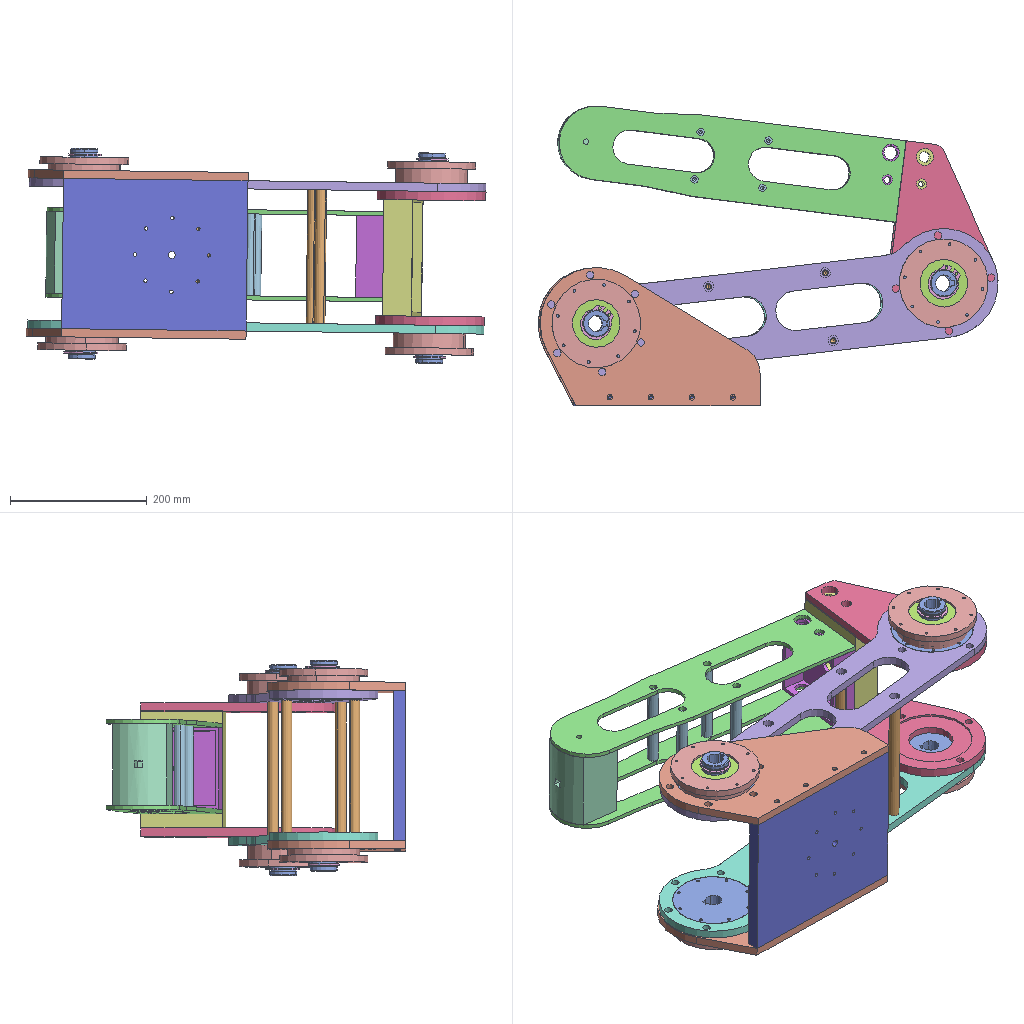Assembly | SolidWorks | 15 different items | 36 placed | box 673 x 438 x 315 mm
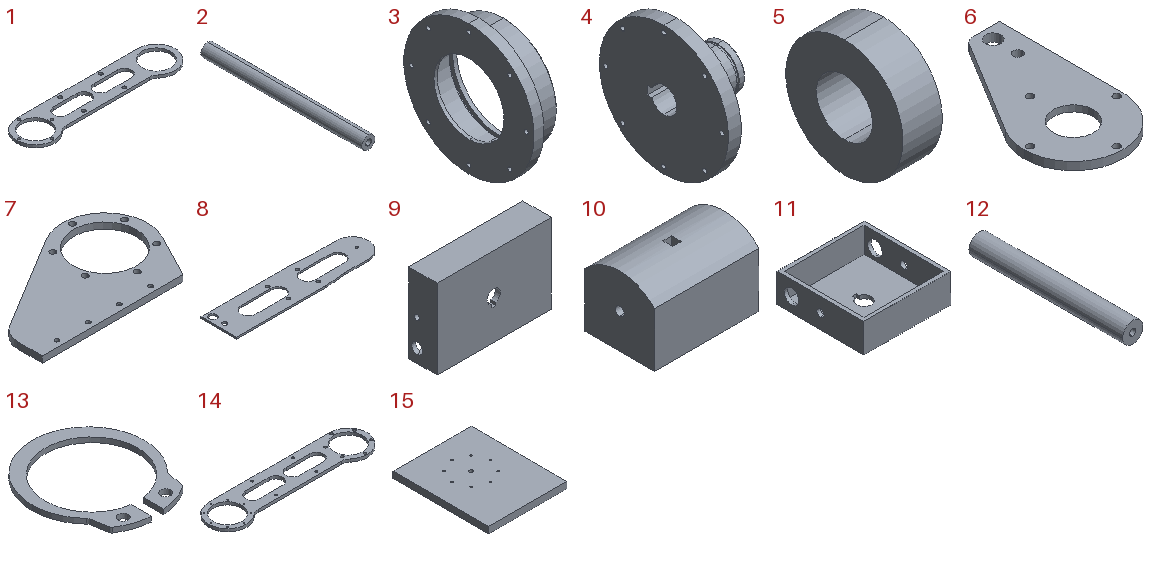Parts list (item | quantity | size | volume | features):
1 | x1 | 672 x 160 x 12 mm | 581826 mm3 | features ICE 4, Extrusion 1, HoleWzd 1
2 | x4 | 16 x 196 x 16 mm | 38778 mm3 | features HoleWzd 2, RevolutionThin 1
3 | x4 | 35 x 130 x 130 mm | 115232 mm3 | features ICE 6, RevolutionThin 2, Chamfer 1
4 | x4 | 56 x 120 x 120 mm | 178131 mm3 | features ICE 3, RevolutionThin 3, Chamfer 1
5 | x4 | 28 x 83.6 x 83.6 mm | 118509 mm3 | features Extrusion 1
6 | x2 | 160 x 280 x 13 mm | 339397 mm3 | features ICE 2, Extrusion 1
7 | x2 | 322 x 202 x 12 mm | 411603 mm3 | features ICE 5, Extrusion 1
8 | x2 | 504 x 120 x 6 mm | 253053 mm3 | features Extrusion 1, HoleWzd 1, ICE 1
9 | x1 | 172 x 42.5 x 120 mm | 233262 mm3 | features ICE 3, Extrusion 1
10 | x1 | 120 x 80 x 80 mm | 704237 mm3 | features ICE 4, Extrusion 1
11 | x1 | 120 x 120 x 40 mm | 146891 mm3 | features ICE 3, Extrusion 1
12 | x4 | 16 x 120 x 16 mm | 23637 mm3 | features HoleWzd 2, RevolutionThin 1
13 | x4 | 45 x 50.322 x 2 mm | 1249 mm3 | features Extrusion 1
14 | x1 | 672 x 160 x 12 mm | 577660 mm3 | features ICE 5, Extrusion 1, HoleWzd 1
15 | x1 | 220 x 270 x 18 mm | 1062194 mm3 | features ICE 5, Extrusion 1
Mates (type | each side: item.copy, entity, surface, feature):
Coincident | 8.1 face plane Boss-Extrude 1 | 12.1 face plane Revolve-Thin 1
Coincident | 8.1 face plane Boss-Extrude 1 | 12.2 face plane Revolve-Thin 1
Coincident | 8.1 face plane Boss-Extrude 1 | 12.3 face plane Revolve-Thin 1
Concentric | 8.1 face cylinder M6 Socket Head CapScrew CounterboreHole 1 | 12.1 face cylinder M6 Tap Drill for Tapped Hole 1
Concentric | 8.1 face cylinder M6 Socket Head CapScrew CounterboreHole 1 | 12.2 face cylinder M6 Tap Drill for Tapped Hole 1
Concentric | 8.1 face cylinder M6 Socket Head CapScrew CounterboreHole 1 | 12.3 face cylinder M6 Tap Drill for Tapped Hole 1
Concentric | 8.2 face cylinder M6 Socket Head CapScrew CounterboreHole 1 | 12.4 face cylinder M6 Tap Drill for Tapped Hole 1
Coincident | 8.1 face plane Boss-Extrude 1 | 12.4 face plane Revolve-Thin 1
Concentric | 14.1 face cylinder M8 Socket Head CapScrew CounterboreHole 2 | 2.1 edge
Concentric | 14.1 face cylinder M8 Socket Head CapScrew CounterboreHole 2 | 2.2 face cylinder M8 Tap Drill for Tapped Hole 2
Concentric | 14.1 face cylinder M8 Socket Head CapScrew CounterboreHole 2 | 2.1 face cylinder M8 Tap Drill for Tapped Hole 1
Concentric | 2.3 edge | 1.1 face cylinder M8 Socket Head CapScrew CounterboreHole 1
Coincident | 2.3 face plane Revolve-Thin 1 | 1.1 face plane Boss-Extrude 2
Concentric | 2.1 face cylinder M8 Tap Drill for Tapped Hole 2 | 1.1 edge
Coincident | 2.1 face plane Revolve-Thin 1 | 1.1 face plane Boss-Extrude 2
Concentric | 2.4 face cone M8 Tap Drill for Tapped Hole 1 | 1.1 edge
Coincident | 2.4 face plane Revolve-Thin 1 | 1.1 face plane Boss-Extrude 2
Concentric | 2.2 edge | 1.1 face cylinder M8 Socket Head CapScrew CounterboreHole 1
Coincident | 2.2 face plane Revolve-Thin 1 | 1.1 face plane Boss-Extrude 2
Coincident | 14.1 face plane Boss-Extrude 2 | 6.1 face plane Boss-Extrude 1
Coincident | 1.1 face plane Boss-Extrude 2 | 6.2 edge
Concentric | 3.1 face cylinder Cut-Extrude 1 | 5.1 face cylinder Boss-Extrude 1
Coincident | 3.1 face plane Cut-Extrude 2 | 5.1 edge
Concentric | 4.1 face cylinder Cut-Extrude 2 | 5.1 face cylinder Boss-Extrude 1
Coincident | 4.1 face plane Revolve-Thin 2 | 5.1 face plane Boss-Extrude 1
Concentric | 4.1 face cylinder Cut-Extrude 2 | 13.1 edge
Coincident | 4.1 face plane Cut-Extrude 4 | 13.1 edge
Concentric | 3.2 face cylinder Cut-Extrude 1 | 5.2 face cylinder Boss-Extrude 1
Coincident | 3.2 face plane Cut-Extrude 2 | 5.2 edge
Concentric | 4.2 face cylinder Cut-Extrude 2 | 5.2 face cylinder Boss-Extrude 1
Coincident | 4.2 face plane Revolve-Thin 2 | 5.2 face plane Boss-Extrude 1
Concentric | 4.2 face cylinder Cut-Extrude 2 | 13.2 edge
Coincident | 4.2 face plane Cut-Extrude 4 | 13.2 edge
Concentric | 4.2 face cylinder Cut-Extrude 2 | 6.1 face cylinder Boss-Extrude 1
Concentric | 4.2 edge | 14.1 edge
Coincident | 4.2 face plane Revolve-Thin 2 | 14.1 face plane Boss-Extrude 2
Concentric | 3.3 face cylinder Cut-Extrude 1 | 5.3 face cylinder Boss-Extrude 1
Coincident | 3.3 face plane Cut-Extrude 2 | 5.3 edge
Concentric | 4.3 face cylinder Cut-Extrude 2 | 5.3 face cylinder Boss-Extrude 1
Coincident | 4.3 face plane Revolve-Thin 2 | 5.3 face plane Boss-Extrude 1
Concentric | 4.3 face cylinder Cut-Extrude 2 | 13.3 edge
Coincident | 4.3 face plane Cut-Extrude 4 | 13.3 edge
Concentric | 4.3 face cylinder Cut-Extrude 2 | 6.2 face cylinder Boss-Extrude 1
Concentric | 4.3 edge | 14.1 face cylinder Boss-Extrude 2
Coincident | 4.3 face plane Revolve-Thin 2 | 1.1 face plane Boss-Extrude 2
Concentric | 3.4 face cylinder Cut-Extrude 1 | 5.4 face cylinder Boss-Extrude 1
Coincident | 3.4 face plane Cut-Extrude 2 | 5.4 edge
Concentric | 4.4 face cylinder Cut-Extrude 2 | 5.4 face cylinder Boss-Extrude 1
Coincident | 4.4 face plane Revolve-Thin 2 | 5.4 face plane Boss-Extrude 1
Concentric | 4.4 face cylinder Cut-Extrude 2 | 13.4 edge
Coincident | 4.4 face plane Cut-Extrude 4 | 13.4 edge
Concentric | 8.2 face cylinder M6 Socket Head CapScrew CounterboreHole 1 | 12.2 face cylinder M6 Tap Drill for Tapped Hole 2
Concentric | 6.2 face cylinder Boss-Extrude 1 | 9.1 face cylinder Cut-Extrude 2 | 2 times
Coincident | 6.1 face plane Boss-Extrude 1 | 9.1 face plane Boss-Extrude 2
Concentric | 6.1 face cylinder Boss-Extrude 1 | 9.1 face cylinder Cut-Extrude 2
Coincident | 8.2 face plane Boss-Extrude 1 | 12.1 face plane Revolve-Thin 1
Concentric | 8.2 edge | 12.1 face cylinder M6 Tap Drill for Tapped Hole 2
Concentric | 8.1 face cylinder Boss-Extrude 1 | 11.1 face cylinder Cut-Extrude 1
Concentric | 8.1 face cylinder Boss-Extrude 1 | 11.1 edge
Coincident | 8.1 face plane Boss-Extrude 1 | 11.1 face plane Boss-Extrude 1
Concentric | 9.1 face cylinder Cut-Extrude 4 | 11.1 face cylinder Cut-Extrude 4
Coincident | 9.1 face plane Boss-Extrude 2 | 11.1 face plane Boss-Extrude 1
Coincident | 14.1 face plane Boss-Extrude 2 | 2.4 edge
Concentric | 4.4 face cylinder Cut-Extrude 2 | 14.1 edge
Concentric | 4.1 face cylinder Cut-Extrude 2 | 1.1 face cylinder Cut-Extrude 2
Parallel | 8.1 edge | 10.1 face plane Boss-Extrude 1
Concentric | 8.2 edge | 10.1 edge
Coincident | 8.2 face plane Boss-Extrude 1 | 10.1 face plane Boss-Extrude 1
Parallel | 1.1 face plane Boss-Extrude 2 | 7.1 edge
Parallel | 7.1 face plane Boss-Extrude 1 | 15.1 face plane Boss-Extrude 1
Concentric | 7.1 edge | 15.1 edge
Coincident | 7.1 face plane Boss-Extrude 1 | 15.1 face plane Boss-Extrude 1
Parallel | 7.2 face plane Boss-Extrude 1 | 15.1 face plane Boss-Extrude 1
Parallel | 7.2 edge | 15.1 face plane Boss-Extrude 1
Concentric | 7.2 face cylinder Cut-Extrude 5 | 15.1 edge
Coincident | 7.2 face plane Boss-Extrude 1 | 15.1 face plane Boss-Extrude 1
Coincident | 4.4 face plane Revolve-Thin 2 | 14.1 face plane Boss-Extrude 2
Coincident | 4.1 face plane Revolve-Thin 2 | 1.1 face plane Boss-Extrude 2
Concentric | 4.4 face cylinder Cut-Extrude 2 | 7.1 face cylinder Cut-Extrude 2
Coincident | 14.1 face plane Boss-Extrude 2 | 7.1 face plane Boss-Extrude 1
Parallel | 9.1 face plane Boss-Extrude 2 | 11.1 face plane Boss-Extrude 1